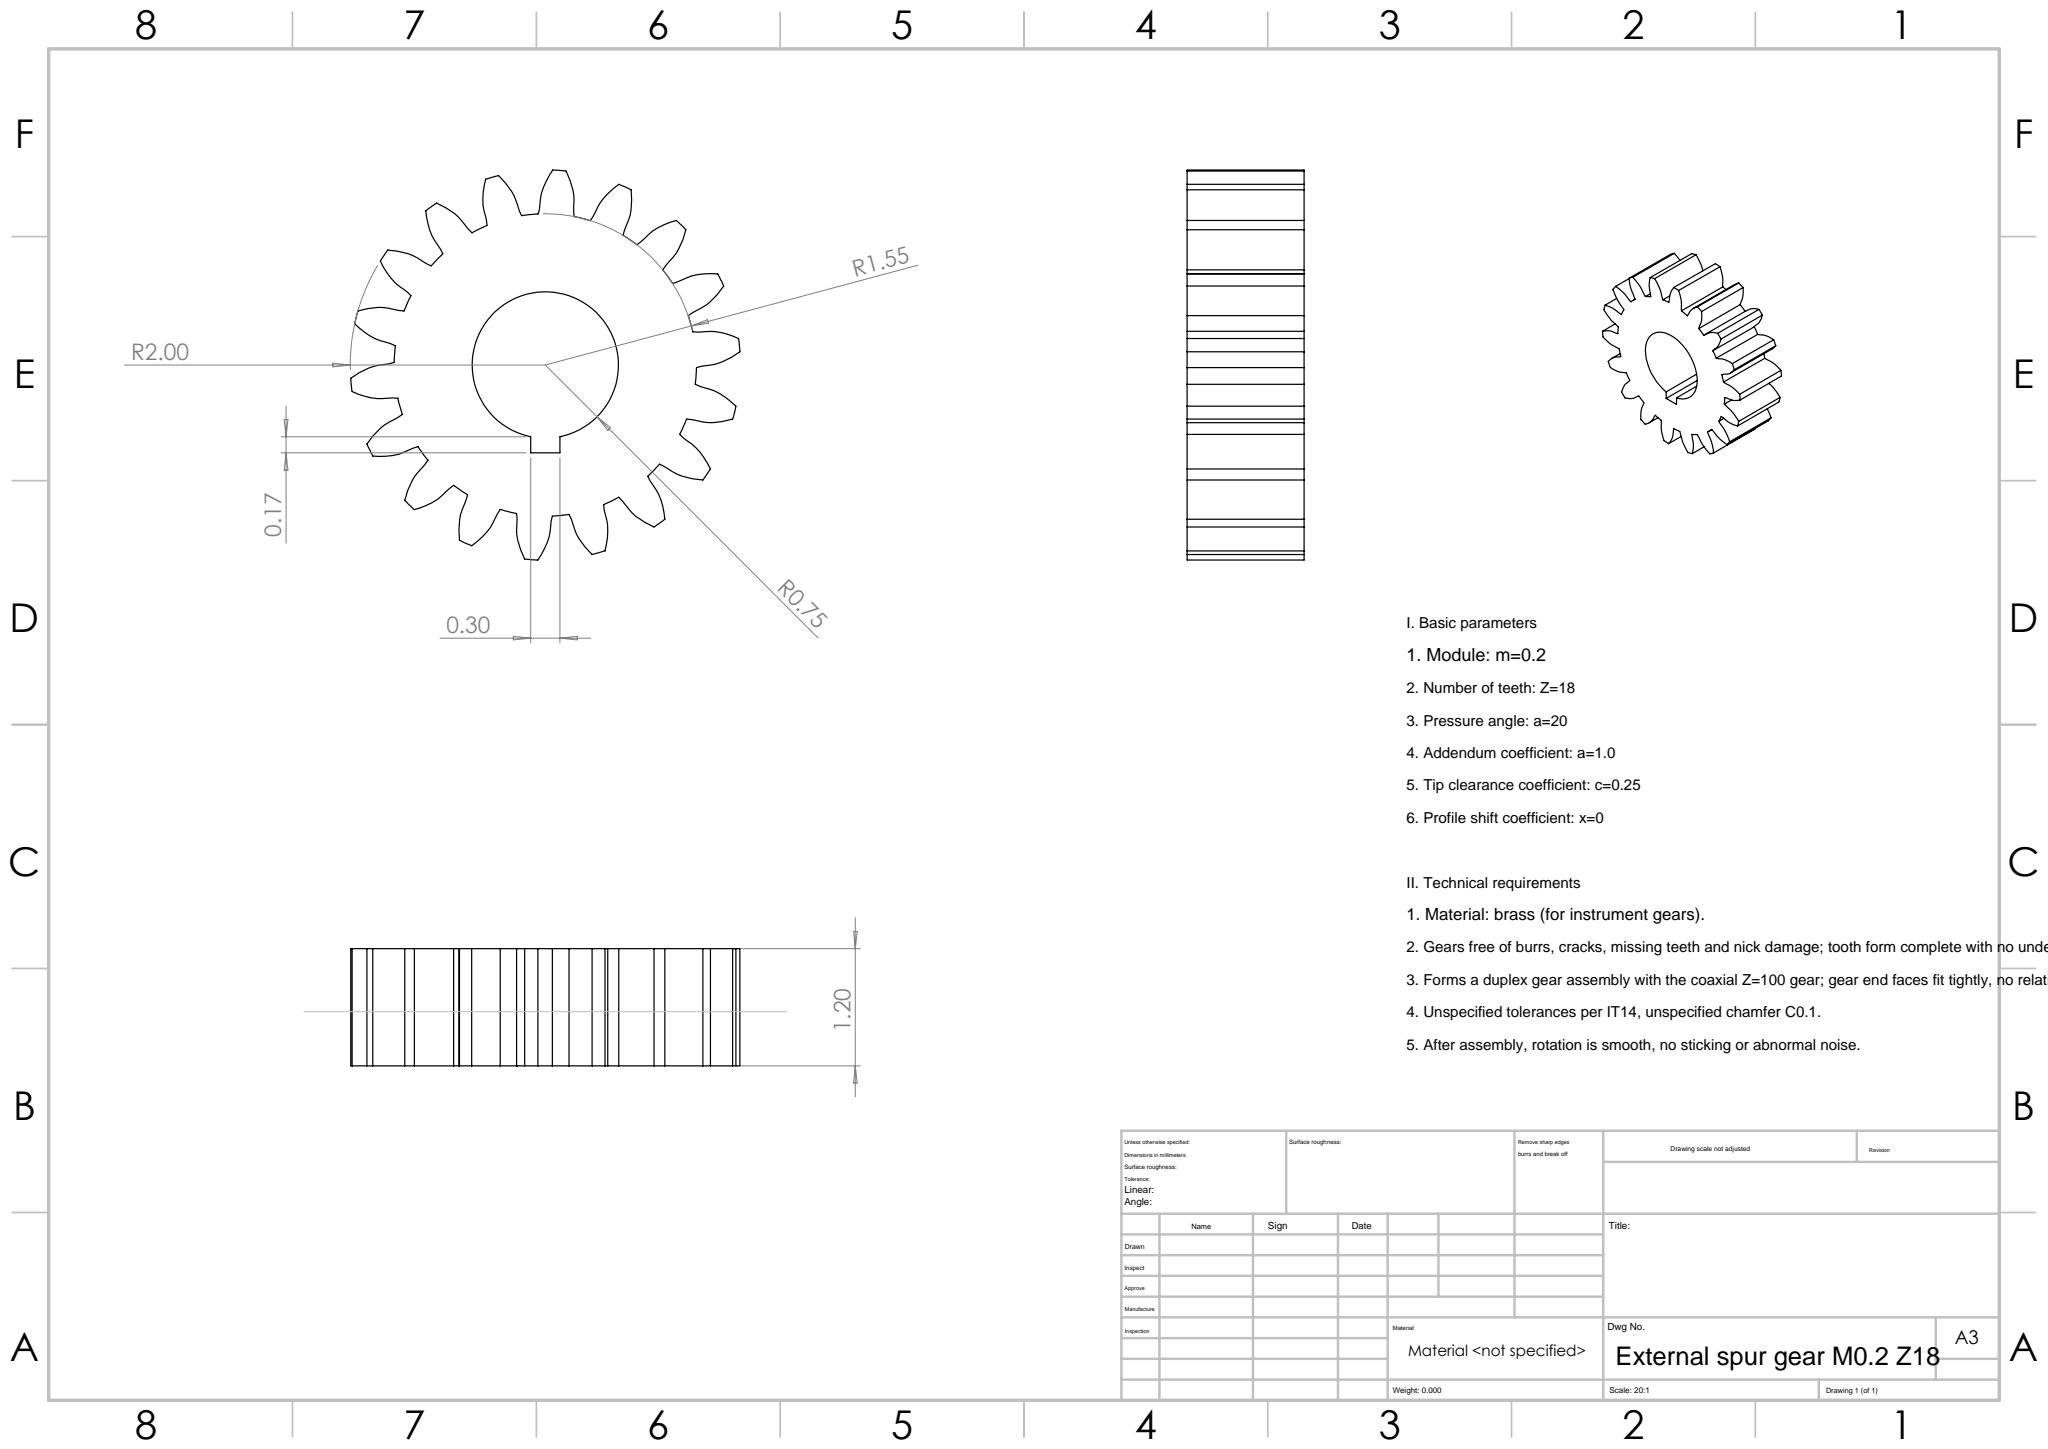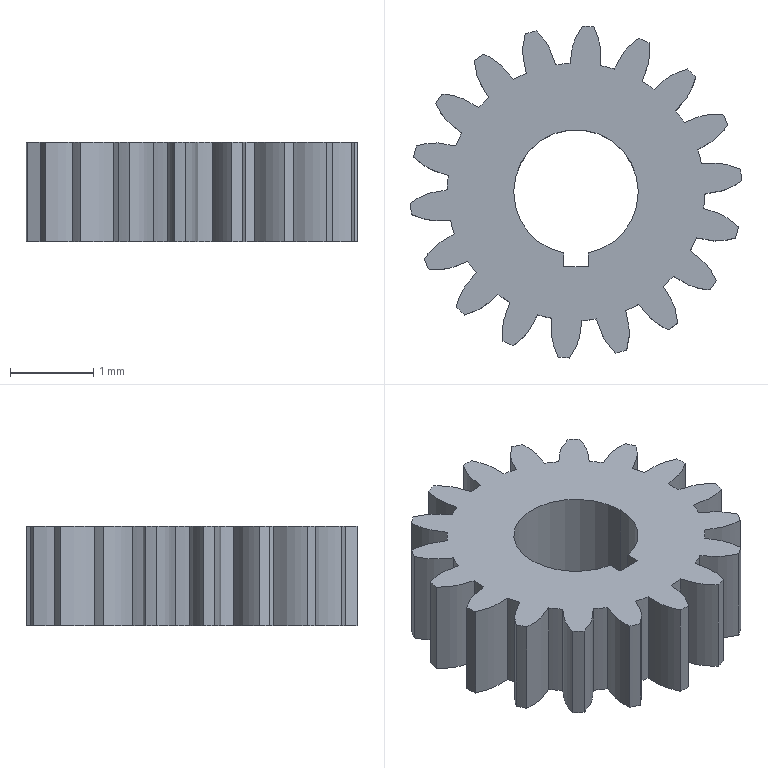Part | SolidWorks | features ICE 2, CirPattern 1, Extrusion 1 | 1 solid | 80 faces | box 3.991 x 3.997 x 1.2 mm | volume 9.749 mm3 | cylinder 39 | spline 36 | plane 5 | commonest cylinder face diameters 3.1 x18 4 x18 1.5 x3